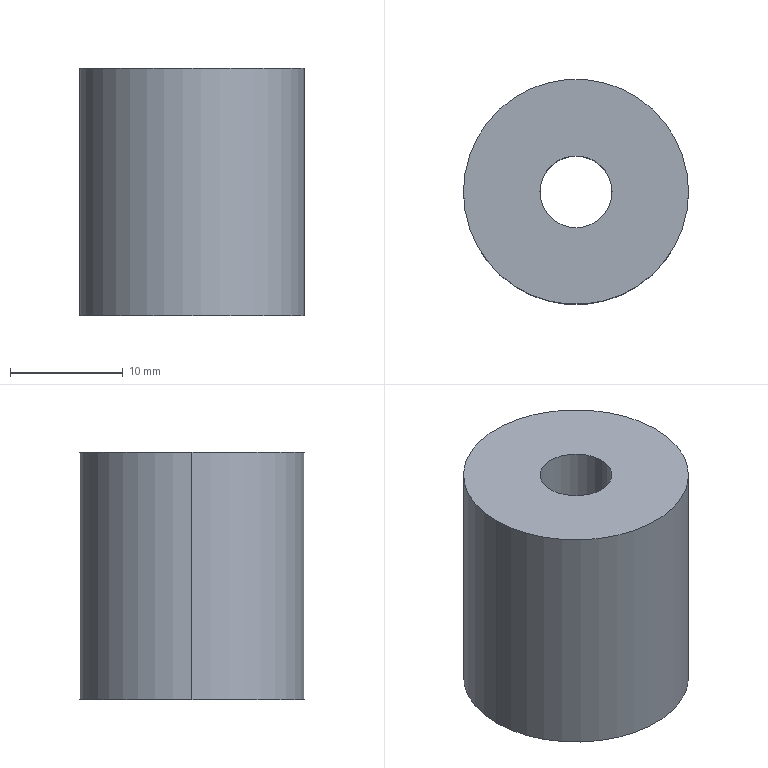Part | SolidWorks | features Extrusion 1 | 1 solid | 6 faces | box 20 x 20 x 22 mm | volume 6204 mm3 | cylinder 4 | plane 2 | commonest cylinder face diameters 6.4 x2 20 x2
STEP:
#1=CARTESIAN_POINT('',(-3.2,0.,-11.));
#2=VERTEX_POINT('',#1);
#3=CARTESIAN_POINT('',(3.2,0.,-11.));
#4=VERTEX_POINT('',#3);
#5=CARTESIAN_POINT('',(0.,0.,-11.));
#6=DIRECTION('',(0.,0.,1.));
#7=DIRECTION('',(1.,0.,0.));
#8=AXIS2_PLACEMENT_3D('',#5,#6,#7);
#9=CIRCLE('',#8,3.2);
#10=EDGE_CURVE('',#2,#4,#9,.T.);
#11=ORIENTED_EDGE('',*,*,#10,.F.);
#12=CARTESIAN_POINT('',(-3.2,0.,11.));
#13=VERTEX_POINT('',#12);
#14=CARTESIAN_POINT('',(-3.2,0.,-11.));
#15=DIRECTION('',(0.,0.,1.));
#16=VECTOR('',#15,1000.);
#17=LINE('',#14,#16);
#18=EDGE_CURVE('',#2,#13,#17,.T.);
#19=ORIENTED_EDGE('',*,*,#18,.T.);
#20=CARTESIAN_POINT('',(3.2,0.,11.));
#21=VERTEX_POINT('',#20);
#22=CARTESIAN_POINT('',(0.,0.,11.));
#23=DIRECTION('',(0.,0.,1.));
#24=DIRECTION('',(1.,0.,0.));
#25=AXIS2_PLACEMENT_3D('',#22,#23,#24);
#26=CIRCLE('',#25,3.2);
#27=EDGE_CURVE('',#13,#21,#26,.T.);
#28=ORIENTED_EDGE('',*,*,#27,.T.);
#29=CARTESIAN_POINT('',(3.2,0.,-11.));
#30=DIRECTION('',(0.,0.,1.));
#31=VECTOR('',#30,1000.);
#32=LINE('',#29,#31);
#33=EDGE_CURVE('',#4,#21,#32,.T.);
#34=ORIENTED_EDGE('',*,*,#33,.F.);
#35=EDGE_LOOP('',(#11,#19,#28,#34));
#36=FACE_OUTER_BOUND('',#35,.T.);
#37=CARTESIAN_POINT('',(0.,0.,-11.));
#38=DIRECTION('',(0.,0.,1.));
#39=DIRECTION('',(1.,0.,0.));
#40=AXIS2_PLACEMENT_3D('',#37,#38,#39);
#41=CYLINDRICAL_SURFACE('',#40,3.2);
#42=ADVANCED_FACE('',(#36),#41,.F.);
#43=CARTESIAN_POINT('',(10.,0.,-11.));
#44=VERTEX_POINT('',#43);
#45=CARTESIAN_POINT('',(-10.,0.,-11.));
#46=VERTEX_POINT('',#45);
#47=CARTESIAN_POINT('',(0.,0.,-11.));
#48=DIRECTION('',(0.,0.,1.));
#49=DIRECTION('',(1.,0.,0.));
#50=AXIS2_PLACEMENT_3D('',#47,#48,#49);
#51=CIRCLE('',#50,10.);
#52=EDGE_CURVE('',#44,#46,#51,.T.);
#53=ORIENTED_EDGE('',*,*,#52,.T.);
#54=CARTESIAN_POINT('',(-10.,0.,11.));
#55=VERTEX_POINT('',#54);
#56=CARTESIAN_POINT('',(-10.,0.,-11.));
#57=DIRECTION('',(0.,0.,1.));
#58=VECTOR('',#57,1000.);
#59=LINE('',#56,#58);
#60=EDGE_CURVE('',#46,#55,#59,.T.);
#61=ORIENTED_EDGE('',*,*,#60,.T.);
#62=CARTESIAN_POINT('',(10.,0.,11.));
#63=VERTEX_POINT('',#62);
#64=CARTESIAN_POINT('',(0.,0.,11.));
#65=DIRECTION('',(0.,0.,1.));
#66=DIRECTION('',(1.,0.,0.));
#67=AXIS2_PLACEMENT_3D('',#64,#65,#66);
#68=CIRCLE('',#67,10.);
#69=EDGE_CURVE('',#63,#55,#68,.T.);
#70=ORIENTED_EDGE('',*,*,#69,.F.);
#71=CARTESIAN_POINT('',(10.,0.,-11.));
#72=DIRECTION('',(0.,0.,1.));
#73=VECTOR('',#72,1000.);
#74=LINE('',#71,#73);
#75=EDGE_CURVE('',#44,#63,#74,.T.);
#76=ORIENTED_EDGE('',*,*,#75,.F.);
#77=EDGE_LOOP('',(#53,#61,#70,#76));
#78=FACE_OUTER_BOUND('',#77,.T.);
#79=CARTESIAN_POINT('',(0.,0.,-11.));
#80=DIRECTION('',(0.,0.,1.));
#81=DIRECTION('',(1.,0.,0.));
#82=AXIS2_PLACEMENT_3D('',#79,#80,#81);
#83=CYLINDRICAL_SURFACE('',#82,10.);
#84=ADVANCED_FACE('',(#78),#83,.T.);
#85=ORIENTED_EDGE('',*,*,#60,.F.);
#86=CARTESIAN_POINT('',(0.,0.,-11.));
#87=DIRECTION('',(0.,0.,1.));
#88=DIRECTION('',(1.,0.,0.));
#89=AXIS2_PLACEMENT_3D('',#86,#87,#88);
#90=CIRCLE('',#89,10.);
#91=EDGE_CURVE('',#46,#44,#90,.T.);
#92=ORIENTED_EDGE('',*,*,#91,.T.);
#93=ORIENTED_EDGE('',*,*,#75,.T.);
#94=CARTESIAN_POINT('',(0.,0.,11.));
#95=DIRECTION('',(0.,0.,1.));
#96=DIRECTION('',(1.,0.,0.));
#97=AXIS2_PLACEMENT_3D('',#94,#95,#96);
#98=CIRCLE('',#97,10.);
#99=EDGE_CURVE('',#55,#63,#98,.T.);
#100=ORIENTED_EDGE('',*,*,#99,.F.);
#101=EDGE_LOOP('',(#85,#92,#93,#100));
#102=FACE_OUTER_BOUND('',#101,.T.);
#103=CARTESIAN_POINT('',(0.,0.,-11.));
#104=DIRECTION('',(0.,0.,1.));
#105=DIRECTION('',(1.,0.,0.));
#106=AXIS2_PLACEMENT_3D('',#103,#104,#105);
#107=CYLINDRICAL_SURFACE('',#106,10.);
#108=ADVANCED_FACE('',(#102),#107,.T.);
#109=CARTESIAN_POINT('',(0.,0.,-11.));
#110=DIRECTION('',(0.,0.,1.));
#111=DIRECTION('',(1.,0.,0.));
#112=AXIS2_PLACEMENT_3D('',#109,#110,#111);
#113=CIRCLE('',#112,3.2);
#114=EDGE_CURVE('',#4,#2,#113,.T.);
#115=ORIENTED_EDGE('',*,*,#114,.T.);
#116=ORIENTED_EDGE('',*,*,#10,.T.);
#117=EDGE_LOOP('',(#115,#116));
#118=FACE_BOUND('',#117,.T.);
#119=ORIENTED_EDGE('',*,*,#52,.F.);
#120=ORIENTED_EDGE('',*,*,#91,.F.);
#121=EDGE_LOOP('',(#119,#120));
#122=FACE_OUTER_BOUND('',#121,.T.);
#123=CARTESIAN_POINT('',(0.,0.,-11.));
#124=DIRECTION('',(0.,0.,1.));
#125=DIRECTION('',(1.,0.,0.));
#126=AXIS2_PLACEMENT_3D('',#123,#124,#125);
#127=PLANE('',#126);
#128=ADVANCED_FACE('',(#118,#122),#127,.F.);
#129=CARTESIAN_POINT('',(0.,0.,11.));
#130=DIRECTION('',(0.,0.,1.));
#131=DIRECTION('',(1.,0.,0.));
#132=AXIS2_PLACEMENT_3D('',#129,#130,#131);
#133=CIRCLE('',#132,3.2);
#134=EDGE_CURVE('',#21,#13,#133,.T.);
#135=ORIENTED_EDGE('',*,*,#134,.F.);
#136=ORIENTED_EDGE('',*,*,#27,.F.);
#137=EDGE_LOOP('',(#135,#136));
#138=FACE_BOUND('',#137,.T.);
#139=ORIENTED_EDGE('',*,*,#69,.T.);
#140=ORIENTED_EDGE('',*,*,#99,.T.);
#141=EDGE_LOOP('',(#139,#140));
#142=FACE_OUTER_BOUND('',#141,.T.);
#143=CARTESIAN_POINT('',(0.,0.,11.));
#144=DIRECTION('',(0.,0.,1.));
#145=DIRECTION('',(1.,0.,0.));
#146=AXIS2_PLACEMENT_3D('',#143,#144,#145);
#147=PLANE('',#146);
#148=ADVANCED_FACE('',(#138,#142),#147,.T.);
#149=ORIENTED_EDGE('',*,*,#18,.F.);
#150=ORIENTED_EDGE('',*,*,#114,.F.);
#151=ORIENTED_EDGE('',*,*,#33,.T.);
#152=ORIENTED_EDGE('',*,*,#134,.T.);
#153=EDGE_LOOP('',(#149,#150,#151,#152));
#154=FACE_OUTER_BOUND('',#153,.T.);
#155=CARTESIAN_POINT('',(0.,0.,-11.));
#156=DIRECTION('',(0.,0.,1.));
#157=DIRECTION('',(1.,0.,0.));
#158=AXIS2_PLACEMENT_3D('',#155,#156,#157);
#159=CYLINDRICAL_SURFACE('',#158,3.2);
#160=ADVANCED_FACE('',(#154),#159,.F.);
#161=CLOSED_SHELL('',(#42,#84,#108,#128,#148,#160));
#162=MANIFOLD_SOLID_BREP('',#161);
#163=CARTESIAN_POINT('',(0.,0.,0.));
#164=DIRECTION('',(0.,0.,1.));
#165=DIRECTION('',(1.,0.,0.));
#166=AXIS2_PLACEMENT_3D('',#163,#164,#165);
#167=(LENGTH_UNIT()NAMED_UNIT(*)SI_UNIT(.MILLI.,.METRE.));
#168=UNCERTAINTY_MEASURE_WITH_UNIT(LENGTH_MEASURE(0.00001),#167,'','');
#169=(NAMED_UNIT(*)PLANE_ANGLE_UNIT()SI_UNIT($,.RADIAN.));
#170=(NAMED_UNIT(*)SI_UNIT($,.STERADIAN.)SOLID_ANGLE_UNIT());
#171=(GEOMETRIC_REPRESENTATION_CONTEXT(3)GLOBAL_UNCERTAINTY_ASSIGNED_CONTEXT((#168))GLOBAL_UNIT_ASSIGNED_CONTEXT((#167,#169,#170))REPRESENTATION_CONTEXT('',''));
#172=ADVANCED_BREP_SHAPE_REPRESENTATION('',(#162,#166),#171);